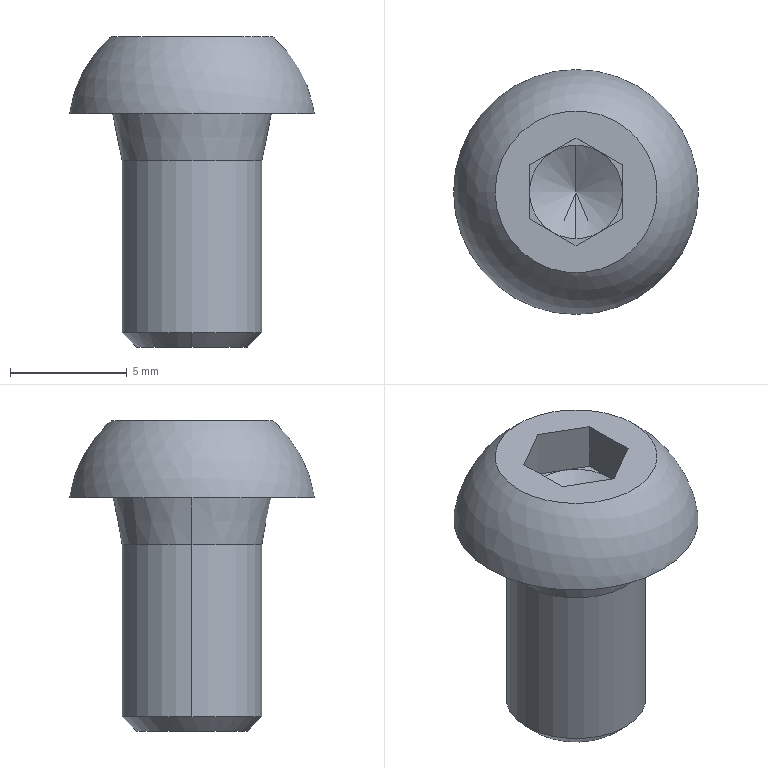Part | SolidWorks | features BaseBody 1 | 1 solid | 24 faces | box 10.5 x 10.5 x 13.3 mm | volume 477.821 mm3 | plane 15 | cone 6 | cylinder 2 | sphere 1 | commonest cylinder face diameters 6 x2
STEP:
#1=CARTESIAN_POINT('',(3.,0.,0.));
#2=VERTEX_POINT('',#1);
#3=CARTESIAN_POINT('',(-3.,0.,0.));
#4=VERTEX_POINT('',#3);
#5=CARTESIAN_POINT('',(0.,0.,0.));
#6=DIRECTION('',(0.,0.,1.));
#7=DIRECTION('',(1.,0.,0.));
#8=AXIS2_PLACEMENT_3D('',#5,#6,#7);
#9=CIRCLE('',#8,3.);
#10=EDGE_CURVE('',#2,#4,#9,.T.);
#11=ORIENTED_EDGE('',*,*,#10,.T.);
#12=CARTESIAN_POINT('',(-3.4,0.,2.));
#13=VERTEX_POINT('',#12);
#14=CARTESIAN_POINT('',(-3.4,0.,2.));
#15=DIRECTION('',(-0.1961,0.,0.9806));
#16=VECTOR('',#15,1000.);
#17=LINE('',#14,#16);
#18=EDGE_CURVE('',#4,#13,#17,.T.);
#19=ORIENTED_EDGE('',*,*,#18,.T.);
#20=CARTESIAN_POINT('',(3.4,0.,2.));
#21=VERTEX_POINT('',#20);
#22=CARTESIAN_POINT('',(0.,0.,2.));
#23=DIRECTION('',(0.,0.,-1.));
#24=DIRECTION('',(1.,0.,0.));
#25=AXIS2_PLACEMENT_3D('',#22,#23,#24);
#26=CIRCLE('',#25,3.4);
#27=EDGE_CURVE('',#13,#21,#26,.T.);
#28=ORIENTED_EDGE('',*,*,#27,.T.);
#29=CARTESIAN_POINT('',(3.4,0.,2.));
#30=DIRECTION('',(0.1961,0.,0.9806));
#31=VECTOR('',#30,1000.);
#32=LINE('',#29,#31);
#33=EDGE_CURVE('',#2,#21,#32,.T.);
#34=ORIENTED_EDGE('',*,*,#33,.F.);
#35=EDGE_LOOP('',(#11,#19,#28,#34));
#36=FACE_OUTER_BOUND('',#35,.T.);
#37=CARTESIAN_POINT('',(0.,0.,2.));
#38=DIRECTION('',(0.,0.,1.));
#39=DIRECTION('',(1.,0.,0.));
#40=AXIS2_PLACEMENT_3D('',#37,#38,#39);
#41=CONICAL_SURFACE('',#40,3.4,0.1974);
#42=ADVANCED_FACE('',(#36),#41,.T.);
#43=CARTESIAN_POINT('',(0.,3.,-7.387));
#44=VERTEX_POINT('',#43);
#45=CARTESIAN_POINT('',(-3.,0.,-7.387));
#46=VERTEX_POINT('',#45);
#47=CARTESIAN_POINT('',(0.,0.,-7.387));
#48=DIRECTION('',(0.,0.,1.));
#49=DIRECTION('',(1.,0.,0.));
#50=AXIS2_PLACEMENT_3D('',#47,#48,#49);
#51=CIRCLE('',#50,3.);
#52=EDGE_CURVE('',#44,#46,#51,.T.);
#53=ORIENTED_EDGE('',*,*,#52,.T.);
#54=CARTESIAN_POINT('',(-3.,0.,-8.));
#55=DIRECTION('',(0.,0.,1.));
#56=VECTOR('',#55,1000.);
#57=LINE('',#54,#56);
#58=EDGE_CURVE('',#46,#4,#57,.T.);
#59=ORIENTED_EDGE('',*,*,#58,.T.);
#60=ORIENTED_EDGE('',*,*,#10,.F.);
#61=CARTESIAN_POINT('',(3.,0.,-7.387));
#62=VERTEX_POINT('',#61);
#63=CARTESIAN_POINT('',(3.,0.,-8.));
#64=DIRECTION('',(0.,0.,1.));
#65=VECTOR('',#64,1000.);
#66=LINE('',#63,#65);
#67=EDGE_CURVE('',#62,#2,#66,.T.);
#68=ORIENTED_EDGE('',*,*,#67,.F.);
#69=CARTESIAN_POINT('',(0.,0.,-7.387));
#70=DIRECTION('',(0.,0.,1.));
#71=DIRECTION('',(1.,0.,0.));
#72=AXIS2_PLACEMENT_3D('',#69,#70,#71);
#73=CIRCLE('',#72,3.);
#74=EDGE_CURVE('',#62,#44,#73,.T.);
#75=ORIENTED_EDGE('',*,*,#74,.T.);
#76=EDGE_LOOP('',(#53,#59,#60,#68,#75));
#77=FACE_OUTER_BOUND('',#76,.T.);
#78=CARTESIAN_POINT('',(0.,0.,-8.));
#79=DIRECTION('',(0.,0.,1.));
#80=DIRECTION('',(1.,0.,0.));
#81=AXIS2_PLACEMENT_3D('',#78,#79,#80);
#82=CYLINDRICAL_SURFACE('',#81,3.);
#83=ADVANCED_FACE('',(#77),#82,.T.);
#84=CARTESIAN_POINT('',(0.,0.,2.065));
#85=VERTEX_POINT('',#84);
#86=CARTESIAN_POINT('',(0.,-2.,3.22));
#87=VERTEX_POINT('',#86);
#88=CARTESIAN_POINT('',(0.,-2.,3.22));
#89=DIRECTION('',(0.,-0.866,0.5));
#90=VECTOR('',#89,1000.);
#91=LINE('',#88,#90);
#92=EDGE_CURVE('',#85,#87,#91,.T.);
#93=ORIENTED_EDGE('',*,*,#92,.F.);
#94=CARTESIAN_POINT('',(0.,2.,3.22));
#95=VERTEX_POINT('',#94);
#96=CARTESIAN_POINT('',(0.,2.,3.22));
#97=DIRECTION('',(0.,0.866,0.5));
#98=VECTOR('',#97,1000.);
#99=LINE('',#96,#98);
#100=EDGE_CURVE('',#85,#95,#99,.T.);
#101=ORIENTED_EDGE('',*,*,#100,.T.);
#102=CARTESIAN_POINT('',(-1.,1.732,3.22));
#103=VERTEX_POINT('',#102);
#104=CARTESIAN_POINT('',(0.,0.,3.22));
#105=DIRECTION('',(0.,0.,-1.));
#106=DIRECTION('',(0.,-1.,0.));
#107=AXIS2_PLACEMENT_3D('',#104,#105,#106);
#108=CIRCLE('',#107,2.);
#109=EDGE_CURVE('',#103,#95,#108,.T.);
#110=ORIENTED_EDGE('',*,*,#109,.F.);
#111=CARTESIAN_POINT('',(-2.,0.,3.22));
#112=VERTEX_POINT('',#111);
#113=CARTESIAN_POINT('',(0.,0.,3.22));
#114=DIRECTION('',(0.,0.,-1.));
#115=DIRECTION('',(0.,-1.,0.));
#116=AXIS2_PLACEMENT_3D('',#113,#114,#115);
#117=CIRCLE('',#116,2.);
#118=EDGE_CURVE('',#112,#103,#117,.T.);
#119=ORIENTED_EDGE('',*,*,#118,.F.);
#120=CARTESIAN_POINT('',(-1.,-1.732,3.22));
#121=VERTEX_POINT('',#120);
#122=CARTESIAN_POINT('',(0.,0.,3.22));
#123=DIRECTION('',(0.,0.,-1.));
#124=DIRECTION('',(0.,-1.,0.));
#125=AXIS2_PLACEMENT_3D('',#122,#123,#124);
#126=CIRCLE('',#125,2.);
#127=EDGE_CURVE('',#121,#112,#126,.T.);
#128=ORIENTED_EDGE('',*,*,#127,.F.);
#129=CARTESIAN_POINT('',(0.,0.,3.22));
#130=DIRECTION('',(0.,0.,-1.));
#131=DIRECTION('',(0.,-1.,0.));
#132=AXIS2_PLACEMENT_3D('',#129,#130,#131);
#133=CIRCLE('',#132,2.);
#134=EDGE_CURVE('',#87,#121,#133,.T.);
#135=ORIENTED_EDGE('',*,*,#134,.F.);
#136=EDGE_LOOP('',(#93,#101,#110,#119,#128,#135));
#137=FACE_OUTER_BOUND('',#136,.T.);
#138=CARTESIAN_POINT('',(0.,0.,3.22));
#139=DIRECTION('',(0.,0.,1.));
#140=DIRECTION('',(0.,-1.,0.));
#141=AXIS2_PLACEMENT_3D('',#138,#139,#140);
#142=CONICAL_SURFACE('',#141,2.,1.047);
#143=ADVANCED_FACE('',(#137),#142,.F.);
#144=CARTESIAN_POINT('',(0.,-2.386,-8.));
#145=VERTEX_POINT('',#144);
#146=CARTESIAN_POINT('',(0.,2.386,-8.));
#147=VERTEX_POINT('',#146);
#148=CARTESIAN_POINT('',(0.,0.,-8.));
#149=DIRECTION('',(0.,0.,1.));
#150=DIRECTION('',(0.,-1.,0.));
#151=AXIS2_PLACEMENT_3D('',#148,#149,#150);
#152=CIRCLE('',#151,2.386);
#153=EDGE_CURVE('',#145,#147,#152,.T.);
#154=ORIENTED_EDGE('',*,*,#153,.T.);
#155=CARTESIAN_POINT('',(0.,3.,-7.386));
#156=DIRECTION('',(0.,0.7071,0.7071));
#157=VECTOR('',#156,1000.);
#158=LINE('',#155,#157);
#159=EDGE_CURVE('',#147,#44,#158,.T.);
#160=ORIENTED_EDGE('',*,*,#159,.T.);
#161=ORIENTED_EDGE('',*,*,#74,.F.);
#162=CARTESIAN_POINT('',(0.,-3.,-7.387));
#163=VERTEX_POINT('',#162);
#164=CARTESIAN_POINT('',(0.,0.,-7.387));
#165=DIRECTION('',(0.,0.,1.));
#166=DIRECTION('',(1.,0.,0.));
#167=AXIS2_PLACEMENT_3D('',#164,#165,#166);
#168=CIRCLE('',#167,3.);
#169=EDGE_CURVE('',#163,#62,#168,.T.);
#170=ORIENTED_EDGE('',*,*,#169,.F.);
#171=CARTESIAN_POINT('',(0.,-3.,-7.386));
#172=DIRECTION('',(0.,-0.7071,0.7071));
#173=VECTOR('',#172,1000.);
#174=LINE('',#171,#173);
#175=EDGE_CURVE('',#145,#163,#174,.T.);
#176=ORIENTED_EDGE('',*,*,#175,.F.);
#177=EDGE_LOOP('',(#154,#160,#161,#170,#176));
#178=FACE_OUTER_BOUND('',#177,.T.);
#179=CARTESIAN_POINT('',(0.,0.,-7.386));
#180=DIRECTION('',(0.,0.,1.));
#181=DIRECTION('',(0.,-1.,0.));
#182=AXIS2_PLACEMENT_3D('',#179,#180,#181);
#183=CONICAL_SURFACE('',#182,3.,0.7854);
#184=ADVANCED_FACE('',(#178),#183,.T.);
#185=CARTESIAN_POINT('',(-3.472,0.,5.3));
#186=VERTEX_POINT('',#185);
#187=CARTESIAN_POINT('',(3.472,0.,5.3));
#188=VERTEX_POINT('',#187);
#189=CARTESIAN_POINT('',(0.,0.,5.3));
#190=DIRECTION('',(0.,0.,-1.));
#191=DIRECTION('',(-1.,0.,0.));
#192=AXIS2_PLACEMENT_3D('',#189,#190,#191);
#193=CIRCLE('',#192,3.472);
#194=EDGE_CURVE('',#186,#188,#193,.T.);
#195=ORIENTED_EDGE('',*,*,#194,.T.);
#196=CARTESIAN_POINT('',(0.,0.,5.3));
#197=DIRECTION('',(0.,0.,-1.));
#198=DIRECTION('',(-1.,0.,0.));
#199=AXIS2_PLACEMENT_3D('',#196,#197,#198);
#200=CIRCLE('',#199,3.472);
#201=EDGE_CURVE('',#188,#186,#200,.T.);
#202=ORIENTED_EDGE('',*,*,#201,.T.);
#203=EDGE_LOOP('',(#195,#202));
#204=FACE_BOUND('',#203,.T.);
#205=CARTESIAN_POINT('',(5.25,0.,2.));
#206=VERTEX_POINT('',#205);
#207=CARTESIAN_POINT('',(-5.25,0.,2.));
#208=VERTEX_POINT('',#207);
#209=CARTESIAN_POINT('',(0.,0.,2.));
#210=DIRECTION('',(0.,0.,1.));
#211=DIRECTION('',(1.,0.,0.));
#212=AXIS2_PLACEMENT_3D('',#209,#210,#211);
#213=CIRCLE('',#212,5.25);
#214=EDGE_CURVE('',#206,#208,#213,.T.);
#215=ORIENTED_EDGE('',*,*,#214,.T.);
#216=CARTESIAN_POINT('',(0.,0.,2.));
#217=DIRECTION('',(0.,0.,1.));
#218=DIRECTION('',(1.,0.,0.));
#219=AXIS2_PLACEMENT_3D('',#216,#217,#218);
#220=CIRCLE('',#219,5.25);
#221=EDGE_CURVE('',#208,#206,#220,.T.);
#222=ORIENTED_EDGE('',*,*,#221,.T.);
#223=EDGE_LOOP('',(#215,#222));
#224=FACE_OUTER_BOUND('',#223,.T.);
#225=CARTESIAN_POINT('',(0.,0.,1.3));
#226=DIRECTION('',(0.115,0.,0.9934));
#227=DIRECTION('',(-0.9934,0.,0.115));
#228=AXIS2_PLACEMENT_3D('',#225,#226,#227);
#229=SPHERICAL_SURFACE('',#228,5.296);
#230=ADVANCED_FACE('',(#204,#224),#229,.T.);
#231=ORIENTED_EDGE('',*,*,#194,.F.);
#232=ORIENTED_EDGE('',*,*,#201,.F.);
#233=EDGE_LOOP('',(#231,#232));
#234=FACE_OUTER_BOUND('',#233,.T.);
#235=CARTESIAN_POINT('',(2.,-1.155,5.3));
#236=VERTEX_POINT('',#235);
#237=CARTESIAN_POINT('',(2.,1.155,5.3));
#238=VERTEX_POINT('',#237);
#239=CARTESIAN_POINT('',(2.,0.,5.3));
#240=DIRECTION('',(0.,1.,0.));
#241=VECTOR('',#240,1000.);
#242=LINE('',#239,#241);
#243=EDGE_CURVE('',#236,#238,#242,.T.);
#244=ORIENTED_EDGE('',*,*,#243,.F.);
#245=CARTESIAN_POINT('',(0.,-2.309,5.3));
#246=VERTEX_POINT('',#245);
#247=CARTESIAN_POINT('',(0.,-2.309,5.3));
#248=DIRECTION('',(0.866,0.5,0.));
#249=VECTOR('',#248,1000.);
#250=LINE('',#247,#249);
#251=EDGE_CURVE('',#246,#236,#250,.T.);
#252=ORIENTED_EDGE('',*,*,#251,.F.);
#253=CARTESIAN_POINT('',(-2.,-1.155,5.3));
#254=VERTEX_POINT('',#253);
#255=CARTESIAN_POINT('',(-2.,-1.155,5.3));
#256=DIRECTION('',(0.866,-0.5,0.));
#257=VECTOR('',#256,1000.);
#258=LINE('',#255,#257);
#259=EDGE_CURVE('',#254,#246,#258,.T.);
#260=ORIENTED_EDGE('',*,*,#259,.F.);
#261=CARTESIAN_POINT('',(-2.,1.155,5.3));
#262=VERTEX_POINT('',#261);
#263=CARTESIAN_POINT('',(-2.,0.,5.3));
#264=DIRECTION('',(0.,-1.,0.));
#265=VECTOR('',#264,1000.);
#266=LINE('',#263,#265);
#267=EDGE_CURVE('',#262,#254,#266,.T.);
#268=ORIENTED_EDGE('',*,*,#267,.F.);
#269=CARTESIAN_POINT('',(0.,2.309,5.3));
#270=VERTEX_POINT('',#269);
#271=CARTESIAN_POINT('',(0.,2.309,5.3));
#272=DIRECTION('',(-0.866,-0.5,0.));
#273=VECTOR('',#272,1000.);
#274=LINE('',#271,#273);
#275=EDGE_CURVE('',#270,#262,#274,.T.);
#276=ORIENTED_EDGE('',*,*,#275,.F.);
#277=CARTESIAN_POINT('',(2.,1.155,5.3));
#278=DIRECTION('',(-0.866,0.5,0.));
#279=VECTOR('',#278,1000.);
#280=LINE('',#277,#279);
#281=EDGE_CURVE('',#238,#270,#280,.T.);
#282=ORIENTED_EDGE('',*,*,#281,.F.);
#283=EDGE_LOOP('',(#244,#252,#260,#268,#276,#282));
#284=FACE_BOUND('',#283,.T.);
#285=CARTESIAN_POINT('',(0.,0.,5.3));
#286=DIRECTION('',(0.,0.,-1.));
#287=DIRECTION('',(-1.,0.,0.));
#288=AXIS2_PLACEMENT_3D('',#285,#286,#287);
#289=PLANE('',#288);
#290=ADVANCED_FACE('',(#234,#284),#289,.F.);
#291=ORIENTED_EDGE('',*,*,#214,.F.);
#292=ORIENTED_EDGE('',*,*,#221,.F.);
#293=EDGE_LOOP('',(#291,#292));
#294=FACE_OUTER_BOUND('',#293,.T.);
#295=CARTESIAN_POINT('',(0.,0.,2.));
#296=DIRECTION('',(0.,0.,-1.));
#297=DIRECTION('',(1.,0.,0.));
#298=AXIS2_PLACEMENT_3D('',#295,#296,#297);
#299=CIRCLE('',#298,3.4);
#300=EDGE_CURVE('',#21,#13,#299,.T.);
#301=ORIENTED_EDGE('',*,*,#300,.F.);
#302=ORIENTED_EDGE('',*,*,#27,.F.);
#303=EDGE_LOOP('',(#301,#302));
#304=FACE_BOUND('',#303,.T.);
#305=CARTESIAN_POINT('',(0.,5.25,2.));
#306=DIRECTION('',(0.,0.,1.));
#307=DIRECTION('',(1.,0.,0.));
#308=AXIS2_PLACEMENT_3D('',#305,#306,#307);
#309=PLANE('',#308);
#310=ADVANCED_FACE('',(#294,#304),#309,.F.);
#311=CARTESIAN_POINT('',(0.,2.309,3.22));
#312=VERTEX_POINT('',#311);
#313=CARTESIAN_POINT('',(0.,2.309,3.22));
#314=DIRECTION('',(0.,0.,1.));
#315=VECTOR('',#314,1000.);
#316=LINE('',#313,#315);
#317=EDGE_CURVE('',#312,#270,#316,.T.);
#318=ORIENTED_EDGE('',*,*,#317,.F.);
#319=CARTESIAN_POINT('',(1.,1.732,3.22));
#320=VERTEX_POINT('',#319);
#321=CARTESIAN_POINT('',(2.,1.155,3.22));
#322=DIRECTION('',(-0.866,0.5,0.));
#323=VECTOR('',#322,1000.);
#324=LINE('',#321,#323);
#325=EDGE_CURVE('',#320,#312,#324,.T.);
#326=ORIENTED_EDGE('',*,*,#325,.F.);
#327=CARTESIAN_POINT('',(2.,1.155,3.22));
#328=VERTEX_POINT('',#327);
#329=CARTESIAN_POINT('',(2.,1.155,3.22));
#330=DIRECTION('',(-0.866,0.5,0.));
#331=VECTOR('',#330,1000.);
#332=LINE('',#329,#331);
#333=EDGE_CURVE('',#328,#320,#332,.T.);
#334=ORIENTED_EDGE('',*,*,#333,.F.);
#335=CARTESIAN_POINT('',(2.,1.155,3.22));
#336=DIRECTION('',(0.,0.,-1.));
#337=VECTOR('',#336,1000.);
#338=LINE('',#335,#337);
#339=EDGE_CURVE('',#238,#328,#338,.T.);
#340=ORIENTED_EDGE('',*,*,#339,.F.);
#341=ORIENTED_EDGE('',*,*,#281,.T.);
#342=EDGE_LOOP('',(#318,#326,#334,#340,#341));
#343=FACE_OUTER_BOUND('',#342,.T.);
#344=CARTESIAN_POINT('',(2.,1.155,3.22));
#345=DIRECTION('',(0.5,0.866,0.));
#346=DIRECTION('',(-0.866,0.5,0.));
#347=AXIS2_PLACEMENT_3D('',#344,#345,#346);
#348=PLANE('',#347);
#349=ADVANCED_FACE('',(#343),#348,.F.);
#350=ORIENTED_EDGE('',*,*,#339,.T.);
#351=CARTESIAN_POINT('',(2.,0.,3.22));
#352=VERTEX_POINT('',#351);
#353=CARTESIAN_POINT('',(2.,0.,3.22));
#354=DIRECTION('',(0.,1.,0.));
#355=VECTOR('',#354,1000.);
#356=LINE('',#353,#355);
#357=EDGE_CURVE('',#352,#328,#356,.T.);
#358=ORIENTED_EDGE('',*,*,#357,.F.);
#359=CARTESIAN_POINT('',(2.,-1.155,3.22));
#360=VERTEX_POINT('',#359);
#361=CARTESIAN_POINT('',(2.,0.,3.22));
#362=DIRECTION('',(0.,1.,0.));
#363=VECTOR('',#362,1000.);
#364=LINE('',#361,#363);
#365=EDGE_CURVE('',#360,#352,#364,.T.);
#366=ORIENTED_EDGE('',*,*,#365,.F.);
#367=CARTESIAN_POINT('',(2.,-1.155,3.22));
#368=DIRECTION('',(0.,0.,-1.));
#369=VECTOR('',#368,1000.);
#370=LINE('',#367,#369);
#371=EDGE_CURVE('',#236,#360,#370,.T.);
#372=ORIENTED_EDGE('',*,*,#371,.F.);
#373=ORIENTED_EDGE('',*,*,#243,.T.);
#374=EDGE_LOOP('',(#350,#358,#366,#372,#373));
#375=FACE_OUTER_BOUND('',#374,.T.);
#376=CARTESIAN_POINT('',(2.,-1.155,3.22));
#377=DIRECTION('',(1.,0.,0.));
#378=DIRECTION('',(0.,0.,-1.));
#379=AXIS2_PLACEMENT_3D('',#376,#377,#378);
#380=PLANE('',#379);
#381=ADVANCED_FACE('',(#375),#380,.F.);
#382=ORIENTED_EDGE('',*,*,#371,.T.);
#383=CARTESIAN_POINT('',(1.,-1.732,3.22));
#384=VERTEX_POINT('',#383);
#385=CARTESIAN_POINT('',(1.,-1.732,3.22));
#386=DIRECTION('',(0.866,0.5,0.));
#387=VECTOR('',#386,1000.);
#388=LINE('',#385,#387);
#389=EDGE_CURVE('',#384,#360,#388,.T.);
#390=ORIENTED_EDGE('',*,*,#389,.F.);
#391=CARTESIAN_POINT('',(0.,-2.309,3.22));
#392=VERTEX_POINT('',#391);
#393=CARTESIAN_POINT('',(0.,-2.309,3.22));
#394=DIRECTION('',(0.866,0.5,0.));
#395=VECTOR('',#394,1000.);
#396=LINE('',#393,#395);
#397=EDGE_CURVE('',#392,#384,#396,.T.);
#398=ORIENTED_EDGE('',*,*,#397,.F.);
#399=CARTESIAN_POINT('',(0.,-2.309,3.22));
#400=DIRECTION('',(0.,0.,-1.));
#401=VECTOR('',#400,1000.);
#402=LINE('',#399,#401);
#403=EDGE_CURVE('',#246,#392,#402,.T.);
#404=ORIENTED_EDGE('',*,*,#403,.F.);
#405=ORIENTED_EDGE('',*,*,#251,.T.);
#406=EDGE_LOOP('',(#382,#390,#398,#404,#405));
#407=FACE_OUTER_BOUND('',#406,.T.);
#408=CARTESIAN_POINT('',(0.,-2.309,3.22));
#409=DIRECTION('',(0.5,-0.866,0.));
#410=DIRECTION('',(0.866,0.5,0.));
#411=AXIS2_PLACEMENT_3D('',#408,#409,#410);
#412=PLANE('',#411);
#413=ADVANCED_FACE('',(#407),#412,.F.);
#414=ORIENTED_EDGE('',*,*,#403,.T.);
#415=CARTESIAN_POINT('',(-2.,-1.155,3.22));
#416=DIRECTION('',(0.866,-0.5,0.));
#417=VECTOR('',#416,1000.);
#418=LINE('',#415,#417);
#419=EDGE_CURVE('',#121,#392,#418,.T.);
#420=ORIENTED_EDGE('',*,*,#419,.F.);
#421=CARTESIAN_POINT('',(-2.,-1.155,3.22));
#422=VERTEX_POINT('',#421);
#423=CARTESIAN_POINT('',(-2.,-1.155,3.22));
#424=DIRECTION('',(0.866,-0.5,0.));
#425=VECTOR('',#424,1000.);
#426=LINE('',#423,#425);
#427=EDGE_CURVE('',#422,#121,#426,.T.);
#428=ORIENTED_EDGE('',*,*,#427,.F.);
#429=CARTESIAN_POINT('',(-2.,-1.155,3.22));
#430=DIRECTION('',(0.,0.,-1.));
#431=VECTOR('',#430,1000.);
#432=LINE('',#429,#431);
#433=EDGE_CURVE('',#254,#422,#432,.T.);
#434=ORIENTED_EDGE('',*,*,#433,.F.);
#435=ORIENTED_EDGE('',*,*,#259,.T.);
#436=EDGE_LOOP('',(#414,#420,#428,#434,#435));
#437=FACE_OUTER_BOUND('',#436,.T.);
#438=CARTESIAN_POINT('',(-2.,-1.155,3.22));
#439=DIRECTION('',(-0.5,-0.866,0.));
#440=DIRECTION('',(0.866,-0.5,0.));
#441=AXIS2_PLACEMENT_3D('',#438,#439,#440);
#442=PLANE('',#441);
#443=ADVANCED_FACE('',(#437),#442,.F.);
#444=ORIENTED_EDGE('',*,*,#433,.T.);
#445=CARTESIAN_POINT('',(-2.,0.,3.22));
#446=DIRECTION('',(0.,-1.,0.));
#447=VECTOR('',#446,1000.);
#448=LINE('',#445,#447);
#449=EDGE_CURVE('',#112,#422,#448,.T.);
#450=ORIENTED_EDGE('',*,*,#449,.F.);
#451=CARTESIAN_POINT('',(-2.,1.155,3.22));
#452=VERTEX_POINT('',#451);
#453=CARTESIAN_POINT('',(-2.,0.,3.22));
#454=DIRECTION('',(0.,-1.,0.));
#455=VECTOR('',#454,1000.);
#456=LINE('',#453,#455);
#457=EDGE_CURVE('',#452,#112,#456,.T.);
#458=ORIENTED_EDGE('',*,*,#457,.F.);
#459=CARTESIAN_POINT('',(-2.,1.155,3.22));
#460=DIRECTION('',(0.,0.,-1.));
#461=VECTOR('',#460,1000.);
#462=LINE('',#459,#461);
#463=EDGE_CURVE('',#262,#452,#462,.T.);
#464=ORIENTED_EDGE('',*,*,#463,.F.);
#465=ORIENTED_EDGE('',*,*,#267,.T.);
#466=EDGE_LOOP('',(#444,#450,#458,#464,#465));
#467=FACE_OUTER_BOUND('',#466,.T.);
#468=CARTESIAN_POINT('',(-2.,1.155,3.22));
#469=DIRECTION('',(-1.,0.,0.));
#470=DIRECTION('',(0.,0.,1.));
#471=AXIS2_PLACEMENT_3D('',#468,#469,#470);
#472=PLANE('',#471);
#473=ADVANCED_FACE('',(#467),#472,.F.);
#474=ORIENTED_EDGE('',*,*,#463,.T.);
#475=CARTESIAN_POINT('',(0.,2.309,3.22));
#476=DIRECTION('',(-0.866,-0.5,0.));
#477=VECTOR('',#476,1000.);
#478=LINE('',#475,#477);
#479=EDGE_CURVE('',#103,#452,#478,.T.);
#480=ORIENTED_EDGE('',*,*,#479,.F.);
#481=CARTESIAN_POINT('',(0.,2.309,3.22));
#482=DIRECTION('',(-0.866,-0.5,0.));
#483=VECTOR('',#482,1000.);
#484=LINE('',#481,#483);
#485=EDGE_CURVE('',#312,#103,#484,.T.);
#486=ORIENTED_EDGE('',*,*,#485,.F.);
#487=ORIENTED_EDGE('',*,*,#317,.T.);
#488=ORIENTED_EDGE('',*,*,#275,.T.);
#489=EDGE_LOOP('',(#474,#480,#486,#487,#488));
#490=FACE_OUTER_BOUND('',#489,.T.);
#491=CARTESIAN_POINT('',(0.,2.309,3.22));
#492=DIRECTION('',(-0.5,0.866,0.));
#493=DIRECTION('',(-0.866,-0.5,0.));
#494=AXIS2_PLACEMENT_3D('',#491,#492,#493);
#495=PLANE('',#494);
#496=ADVANCED_FACE('',(#490),#495,.F.);
#497=ORIENTED_EDGE('',*,*,#18,.F.);
#498=CARTESIAN_POINT('',(0.,0.,0.));
#499=DIRECTION('',(0.,0.,1.));
#500=DIRECTION('',(1.,0.,0.));
#501=AXIS2_PLACEMENT_3D('',#498,#499,#500);
#502=CIRCLE('',#501,3.);
#503=EDGE_CURVE('',#4,#2,#502,.T.);
#504=ORIENTED_EDGE('',*,*,#503,.T.);
#505=ORIENTED_EDGE('',*,*,#33,.T.);
#506=ORIENTED_EDGE('',*,*,#300,.T.);
#507=EDGE_LOOP('',(#497,#504,#505,#506));
#508=FACE_OUTER_BOUND('',#507,.T.);
#509=CARTESIAN_POINT('',(0.,0.,2.));
#510=DIRECTION('',(0.,0.,1.));
#511=DIRECTION('',(1.,0.,0.));
#512=AXIS2_PLACEMENT_3D('',#509,#510,#511);
#513=CONICAL_SURFACE('',#512,3.4,0.1974);
#514=ADVANCED_FACE('',(#508),#513,.T.);
#515=ORIENTED_EDGE('',*,*,#109,.T.);
#516=CARTESIAN_POINT('',(0.,0.,3.22));
#517=DIRECTION('',(0.,0.,-1.));
#518=DIRECTION('',(0.,-1.,0.));
#519=AXIS2_PLACEMENT_3D('',#516,#517,#518);
#520=CIRCLE('',#519,2.);
#521=EDGE_CURVE('',#95,#320,#520,.T.);
#522=ORIENTED_EDGE('',*,*,#521,.T.);
#523=ORIENTED_EDGE('',*,*,#325,.T.);
#524=ORIENTED_EDGE('',*,*,#485,.T.);
#525=EDGE_LOOP('',(#515,#522,#523,#524));
#526=FACE_OUTER_BOUND('',#525,.T.);
#527=CARTESIAN_POINT('',(0.,0.,3.22));
#528=DIRECTION('',(0.,0.,1.));
#529=DIRECTION('',(1.,0.,0.));
#530=AXIS2_PLACEMENT_3D('',#527,#528,#529);
#531=PLANE('',#530);
#532=ADVANCED_FACE('',(#526),#531,.T.);
#533=CARTESIAN_POINT('',(0.,0.,3.22));
#534=DIRECTION('',(0.,0.,-1.));
#535=DIRECTION('',(0.,-1.,0.));
#536=AXIS2_PLACEMENT_3D('',#533,#534,#535);
#537=CIRCLE('',#536,2.);
#538=EDGE_CURVE('',#384,#87,#537,.T.);
#539=ORIENTED_EDGE('',*,*,#538,.T.);
#540=ORIENTED_EDGE('',*,*,#134,.T.);
#541=ORIENTED_EDGE('',*,*,#419,.T.);
#542=ORIENTED_EDGE('',*,*,#397,.T.);
#543=EDGE_LOOP('',(#539,#540,#541,#542));
#544=FACE_OUTER_BOUND('',#543,.T.);
#545=CARTESIAN_POINT('',(0.,0.,3.22));
#546=DIRECTION('',(0.,0.,1.));
#547=DIRECTION('',(1.,0.,0.));
#548=AXIS2_PLACEMENT_3D('',#545,#546,#547);
#549=PLANE('',#548);
#550=ADVANCED_FACE('',(#544),#549,.T.);
#551=ORIENTED_EDGE('',*,*,#118,.T.);
#552=ORIENTED_EDGE('',*,*,#479,.T.);
#553=ORIENTED_EDGE('',*,*,#457,.T.);
#554=EDGE_LOOP('',(#551,#552,#553));
#555=FACE_OUTER_BOUND('',#554,.T.);
#556=CARTESIAN_POINT('',(0.,0.,3.22));
#557=DIRECTION('',(0.,0.,1.));
#558=DIRECTION('',(1.,0.,0.));
#559=AXIS2_PLACEMENT_3D('',#556,#557,#558);
#560=PLANE('',#559);
#561=ADVANCED_FACE('',(#555),#560,.T.);
#562=ORIENTED_EDGE('',*,*,#58,.F.);
#563=CARTESIAN_POINT('',(0.,0.,-7.387));
#564=DIRECTION('',(0.,0.,1.));
#565=DIRECTION('',(1.,0.,0.));
#566=AXIS2_PLACEMENT_3D('',#563,#564,#565);
#567=CIRCLE('',#566,3.);
#568=EDGE_CURVE('',#46,#163,#567,.T.);
#569=ORIENTED_EDGE('',*,*,#568,.T.);
#570=ORIENTED_EDGE('',*,*,#169,.T.);
#571=ORIENTED_EDGE('',*,*,#67,.T.);
#572=ORIENTED_EDGE('',*,*,#503,.F.);
#573=EDGE_LOOP('',(#562,#569,#570,#571,#572));
#574=FACE_OUTER_BOUND('',#573,.T.);
#575=CARTESIAN_POINT('',(0.,0.,-8.));
#576=DIRECTION('',(0.,0.,1.));
#577=DIRECTION('',(1.,0.,0.));
#578=AXIS2_PLACEMENT_3D('',#575,#576,#577);
#579=CYLINDRICAL_SURFACE('',#578,3.);
#580=ADVANCED_FACE('',(#574),#579,.T.);
#581=ORIENTED_EDGE('',*,*,#100,.F.);
#582=ORIENTED_EDGE('',*,*,#92,.T.);
#583=ORIENTED_EDGE('',*,*,#538,.F.);
#584=CARTESIAN_POINT('',(0.,0.,3.22));
#585=DIRECTION('',(0.,0.,-1.));
#586=DIRECTION('',(0.,-1.,0.));
#587=AXIS2_PLACEMENT_3D('',#584,#585,#586);
#588=CIRCLE('',#587,2.);
#589=EDGE_CURVE('',#352,#384,#588,.T.);
#590=ORIENTED_EDGE('',*,*,#589,.F.);
#591=CARTESIAN_POINT('',(0.,0.,3.22));
#592=DIRECTION('',(0.,0.,-1.));
#593=DIRECTION('',(0.,-1.,0.));
#594=AXIS2_PLACEMENT_3D('',#591,#592,#593);
#595=CIRCLE('',#594,2.);
#596=EDGE_CURVE('',#320,#352,#595,.T.);
#597=ORIENTED_EDGE('',*,*,#596,.F.);
#598=ORIENTED_EDGE('',*,*,#521,.F.);
#599=EDGE_LOOP('',(#581,#582,#583,#590,#597,#598));
#600=FACE_OUTER_BOUND('',#599,.T.);
#601=CARTESIAN_POINT('',(0.,0.,3.22));
#602=DIRECTION('',(0.,0.,1.));
#603=DIRECTION('',(0.,-1.,0.));
#604=AXIS2_PLACEMENT_3D('',#601,#602,#603);
#605=CONICAL_SURFACE('',#604,2.,1.047);
#606=ADVANCED_FACE('',(#600),#605,.F.);
#607=ORIENTED_EDGE('',*,*,#159,.F.);
#608=CARTESIAN_POINT('',(0.,0.,-8.));
#609=DIRECTION('',(0.,0.,1.));
#610=DIRECTION('',(0.,-1.,0.));
#611=AXIS2_PLACEMENT_3D('',#608,#609,#610);
#612=CIRCLE('',#611,2.386);
#613=EDGE_CURVE('',#147,#145,#612,.T.);
#614=ORIENTED_EDGE('',*,*,#613,.T.);
#615=ORIENTED_EDGE('',*,*,#175,.T.);
#616=ORIENTED_EDGE('',*,*,#568,.F.);
#617=ORIENTED_EDGE('',*,*,#52,.F.);
#618=EDGE_LOOP('',(#607,#614,#615,#616,#617));
#619=FACE_OUTER_BOUND('',#618,.T.);
#620=CARTESIAN_POINT('',(0.,0.,-7.386));
#621=DIRECTION('',(0.,0.,1.));
#622=DIRECTION('',(0.,-1.,0.));
#623=AXIS2_PLACEMENT_3D('',#620,#621,#622);
#624=CONICAL_SURFACE('',#623,3.,0.7854);
#625=ADVANCED_FACE('',(#619),#624,.T.);
#626=ORIENTED_EDGE('',*,*,#127,.T.);
#627=ORIENTED_EDGE('',*,*,#449,.T.);
#628=ORIENTED_EDGE('',*,*,#427,.T.);
#629=EDGE_LOOP('',(#626,#627,#628));
#630=FACE_OUTER_BOUND('',#629,.T.);
#631=CARTESIAN_POINT('',(0.,0.,3.22));
#632=DIRECTION('',(0.,0.,1.));
#633=DIRECTION('',(1.,0.,0.));
#634=AXIS2_PLACEMENT_3D('',#631,#632,#633);
#635=PLANE('',#634);
#636=ADVANCED_FACE('',(#630),#635,.T.);
#637=ORIENTED_EDGE('',*,*,#153,.F.);
#638=ORIENTED_EDGE('',*,*,#613,.F.);
#639=EDGE_LOOP('',(#637,#638));
#640=FACE_OUTER_BOUND('',#639,.T.);
#641=CARTESIAN_POINT('',(3.,0.,-8.));
#642=DIRECTION('',(0.,0.,-1.));
#643=DIRECTION('',(-1.,0.,0.));
#644=AXIS2_PLACEMENT_3D('',#641,#642,#643);
#645=PLANE('',#644);
#646=ADVANCED_FACE('',(#640),#645,.T.);
#647=ORIENTED_EDGE('',*,*,#589,.T.);
#648=ORIENTED_EDGE('',*,*,#389,.T.);
#649=ORIENTED_EDGE('',*,*,#365,.T.);
#650=EDGE_LOOP('',(#647,#648,#649));
#651=FACE_OUTER_BOUND('',#650,.T.);
#652=CARTESIAN_POINT('',(0.,0.,3.22));
#653=DIRECTION('',(0.,0.,1.));
#654=DIRECTION('',(1.,0.,0.));
#655=AXIS2_PLACEMENT_3D('',#652,#653,#654);
#656=PLANE('',#655);
#657=ADVANCED_FACE('',(#651),#656,.T.);
#658=ORIENTED_EDGE('',*,*,#596,.T.);
#659=ORIENTED_EDGE('',*,*,#357,.T.);
#660=ORIENTED_EDGE('',*,*,#333,.T.);
#661=EDGE_LOOP('',(#658,#659,#660));
#662=FACE_OUTER_BOUND('',#661,.T.);
#663=CARTESIAN_POINT('',(0.,0.,3.22));
#664=DIRECTION('',(0.,0.,1.));
#665=DIRECTION('',(1.,0.,0.));
#666=AXIS2_PLACEMENT_3D('',#663,#664,#665);
#667=PLANE('',#666);
#668=ADVANCED_FACE('',(#662),#667,.T.);
#669=CLOSED_SHELL('',(#42,#83,#143,#184,#230,#290,#310,#349,#381,#413,#443,#473,#496,#514,#532,#550,#561,#580,#606,#625,#636,#646,#657,#668));
#670=MANIFOLD_SOLID_BREP('',#669);
#671=CARTESIAN_POINT('',(0.,0.,0.));
#672=DIRECTION('',(0.,0.,1.));
#673=DIRECTION('',(1.,0.,0.));
#674=AXIS2_PLACEMENT_3D('',#671,#672,#673);
#675=(LENGTH_UNIT()NAMED_UNIT(*)SI_UNIT(.MILLI.,.METRE.));
#676=UNCERTAINTY_MEASURE_WITH_UNIT(LENGTH_MEASURE(0.00001),#675,'','');
#677=(NAMED_UNIT(*)PLANE_ANGLE_UNIT()SI_UNIT($,.RADIAN.));
#678=(NAMED_UNIT(*)SI_UNIT($,.STERADIAN.)SOLID_ANGLE_UNIT());
#679=(GEOMETRIC_REPRESENTATION_CONTEXT(3)GLOBAL_UNCERTAINTY_ASSIGNED_CONTEXT((#676))GLOBAL_UNIT_ASSIGNED_CONTEXT((#675,#677,#678))REPRESENTATION_CONTEXT('',''));
#680=ADVANCED_BREP_SHAPE_REPRESENTATION('',(#670,#674),#679);